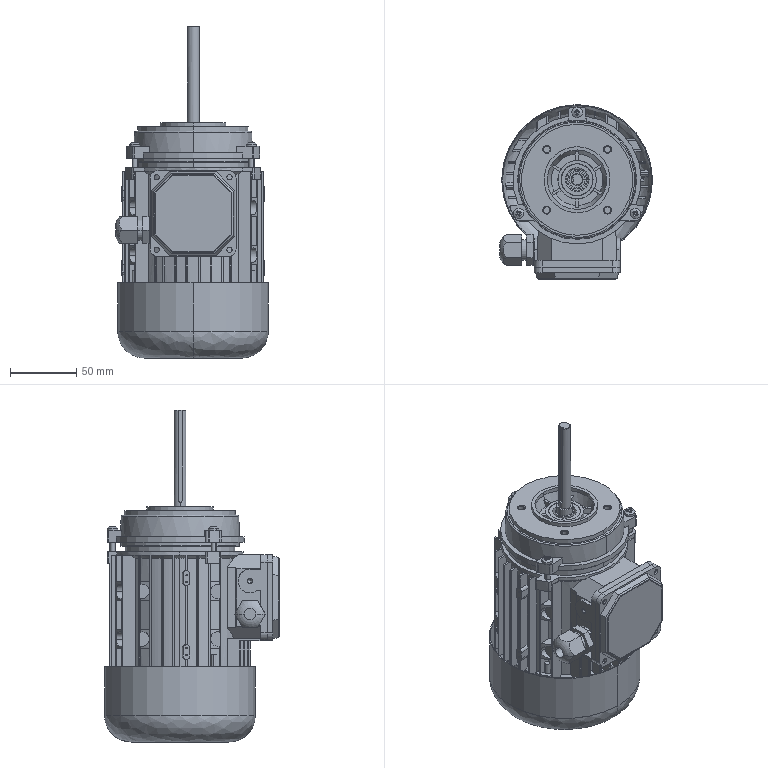Part | SolidWorks | 38 solids | 1742 faces | box 115.663 x 132.2 x 251 mm | volume 733255 mm3 | plane 848 | cylinder 601 | cone 172 | spline 119 | torus 2 | commonest cylinder face diameters 0.4 x88 4 x76 107 x60 92 x46 5 x28 1.6 x26